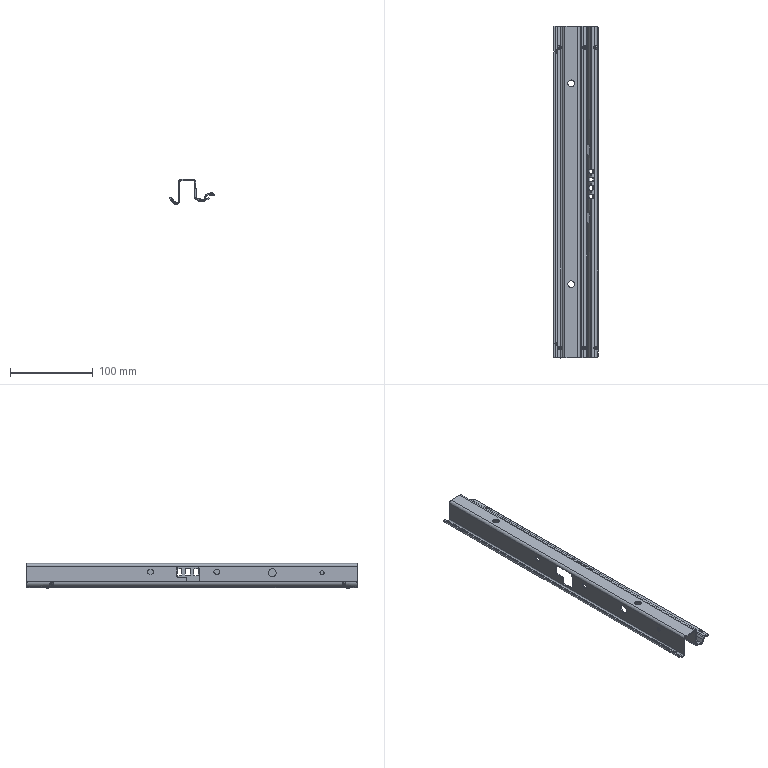Part | 1 solid | 685 faces | box 53.142 x 400 x 30.23 mm | volume 64913 mm3 | spline 234 | cylinder 188 | plane 161 | torus 56 | other 34 | cone 12 | commonest cylinder face diameters 2 x17 0.6 x16 3.7 x16 6 x14 2.9 x12 3.8 x12